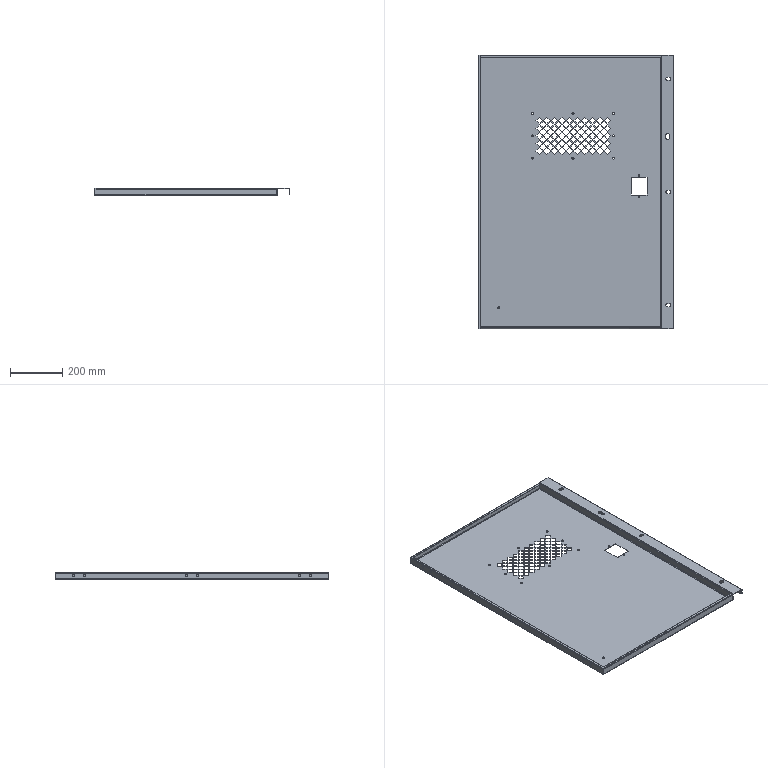Part | STEP file | Rear lower door (upper/lower interlock) | 1 solid | 495 faces | box 748.5 x 1045 x 28 mm | volume 1316932 mm3 | plane 432 | cylinder 63 | commonest cylinder face diameters 7.77 x18 9 x12 13 x11 3 x9 6 x9 5.3 x4